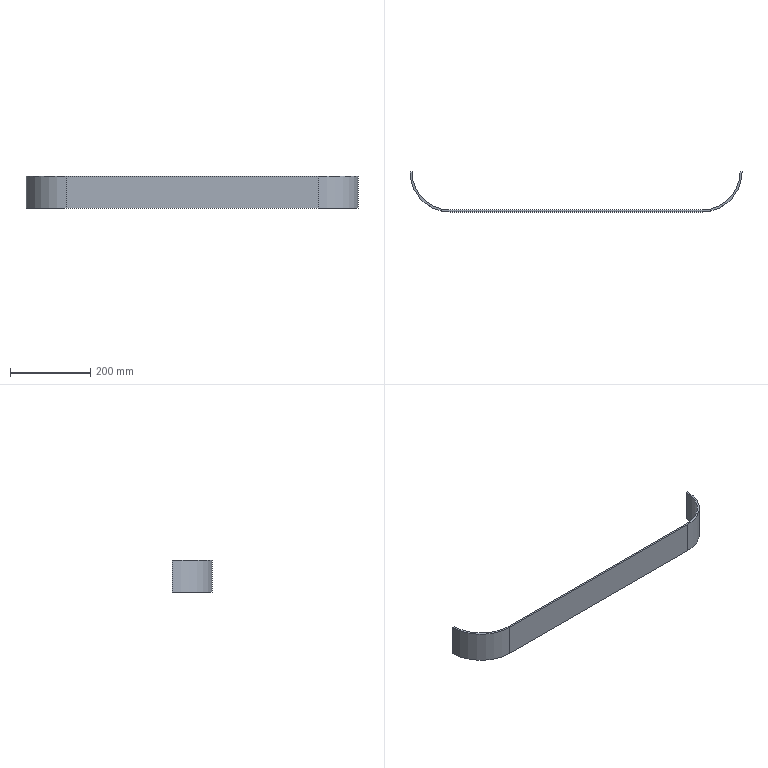Part | NX | features BREP 1 | 1 solid | 10 faces | box 830 x 100 x 80 mm | volume 374522 mm3 | plane 6 | cylinder 4 | commonest cylinder face diameters 190 x2 200 x2
STEP:
#1=CARTESIAN_POINT('',(-315.,-5.,80.));
#2=VERTEX_POINT('',#1);
#3=CARTESIAN_POINT('',(-415.,95.,80.));
#4=VERTEX_POINT('',#3);
#5=CARTESIAN_POINT('',(-315.,95.,80.));
#6=DIRECTION('',(0.,0.,-1.));
#7=DIRECTION('',(1.,0.,0.));
#8=AXIS2_PLACEMENT_3D('',#5,#6,#7);
#9=CIRCLE('',#8,100.);
#10=EDGE_CURVE('',#2,#4,#9,.T.);
#11=ORIENTED_EDGE('',*,*,#10,.F.);
#12=CARTESIAN_POINT('',(315.,-5.,80.));
#13=VERTEX_POINT('',#12);
#14=CARTESIAN_POINT('',(-315.,-5.,80.));
#15=DIRECTION('',(-1.,0.,0.));
#16=VECTOR('',#15,1000.);
#17=LINE('',#14,#16);
#18=EDGE_CURVE('',#13,#2,#17,.T.);
#19=ORIENTED_EDGE('',*,*,#18,.F.);
#20=CARTESIAN_POINT('',(415.,95.,80.));
#21=VERTEX_POINT('',#20);
#22=CARTESIAN_POINT('',(315.,95.,80.));
#23=DIRECTION('',(0.,0.,-1.));
#24=DIRECTION('',(1.,0.,0.));
#25=AXIS2_PLACEMENT_3D('',#22,#23,#24);
#26=CIRCLE('',#25,100.);
#27=EDGE_CURVE('',#21,#13,#26,.T.);
#28=ORIENTED_EDGE('',*,*,#27,.F.);
#29=CARTESIAN_POINT('',(410.,95.,80.));
#30=VERTEX_POINT('',#29);
#31=CARTESIAN_POINT('',(410.,95.,80.));
#32=DIRECTION('',(1.,0.,0.));
#33=VECTOR('',#32,1000.);
#34=LINE('',#31,#33);
#35=EDGE_CURVE('',#30,#21,#34,.T.);
#36=ORIENTED_EDGE('',*,*,#35,.F.);
#37=CARTESIAN_POINT('',(315.,0.,80.));
#38=VERTEX_POINT('',#37);
#39=CARTESIAN_POINT('',(315.,95.,80.));
#40=DIRECTION('',(0.,0.,-1.));
#41=DIRECTION('',(-1.,0.,0.));
#42=AXIS2_PLACEMENT_3D('',#39,#40,#41);
#43=CIRCLE('',#42,95.);
#44=EDGE_CURVE('',#30,#38,#43,.T.);
#45=ORIENTED_EDGE('',*,*,#44,.T.);
#46=CARTESIAN_POINT('',(-315.,0.,80.));
#47=VERTEX_POINT('',#46);
#48=CARTESIAN_POINT('',(-315.,0.,80.));
#49=DIRECTION('',(-1.,0.,0.));
#50=VECTOR('',#49,1000.);
#51=LINE('',#48,#50);
#52=EDGE_CURVE('',#38,#47,#51,.T.);
#53=ORIENTED_EDGE('',*,*,#52,.T.);
#54=CARTESIAN_POINT('',(-410.,95.,80.));
#55=VERTEX_POINT('',#54);
#56=CARTESIAN_POINT('',(-315.,95.,80.));
#57=DIRECTION('',(0.,0.,-1.));
#58=DIRECTION('',(1.,0.,0.));
#59=AXIS2_PLACEMENT_3D('',#56,#57,#58);
#60=CIRCLE('',#59,95.);
#61=EDGE_CURVE('',#47,#55,#60,.T.);
#62=ORIENTED_EDGE('',*,*,#61,.T.);
#63=CARTESIAN_POINT('',(-415.,95.,80.));
#64=DIRECTION('',(1.,0.,0.));
#65=VECTOR('',#64,1000.);
#66=LINE('',#63,#65);
#67=EDGE_CURVE('',#4,#55,#66,.T.);
#68=ORIENTED_EDGE('',*,*,#67,.F.);
#69=EDGE_LOOP('',(#11,#19,#28,#36,#45,#53,#62,#68));
#70=FACE_BOUND('',#69,.T.);
#71=CARTESIAN_POINT('',(-315.,0.,80.));
#72=DIRECTION('',(0.,0.,1.));
#73=DIRECTION('',(1.,0.,0.));
#74=AXIS2_PLACEMENT_3D('',#71,#72,#73);
#75=PLANE('',#74);
#76=ADVANCED_FACE('',(#70),#75,.T.);
#77=CARTESIAN_POINT('',(-315.,0.,0.));
#78=VERTEX_POINT('',#77);
#79=CARTESIAN_POINT('',(-410.,95.,0.));
#80=VERTEX_POINT('',#79);
#81=CARTESIAN_POINT('',(-315.,95.,0.));
#82=DIRECTION('',(0.,0.,-1.));
#83=DIRECTION('',(1.,0.,0.));
#84=AXIS2_PLACEMENT_3D('',#81,#82,#83);
#85=CIRCLE('',#84,95.);
#86=EDGE_CURVE('',#78,#80,#85,.T.);
#87=ORIENTED_EDGE('',*,*,#86,.F.);
#88=CARTESIAN_POINT('',(315.,0.,0.));
#89=VERTEX_POINT('',#88);
#90=CARTESIAN_POINT('',(-315.,0.,0.));
#91=DIRECTION('',(-1.,0.,0.));
#92=VECTOR('',#91,1000.);
#93=LINE('',#90,#92);
#94=EDGE_CURVE('',#89,#78,#93,.T.);
#95=ORIENTED_EDGE('',*,*,#94,.F.);
#96=CARTESIAN_POINT('',(410.,95.,0.));
#97=VERTEX_POINT('',#96);
#98=CARTESIAN_POINT('',(315.,95.,0.));
#99=DIRECTION('',(0.,0.,-1.));
#100=DIRECTION('',(-1.,0.,0.));
#101=AXIS2_PLACEMENT_3D('',#98,#99,#100);
#102=CIRCLE('',#101,95.);
#103=EDGE_CURVE('',#97,#89,#102,.T.);
#104=ORIENTED_EDGE('',*,*,#103,.F.);
#105=CARTESIAN_POINT('',(415.,95.,0.));
#106=VERTEX_POINT('',#105);
#107=CARTESIAN_POINT('',(410.,95.,0.));
#108=DIRECTION('',(1.,0.,0.));
#109=VECTOR('',#108,1000.);
#110=LINE('',#107,#109);
#111=EDGE_CURVE('',#97,#106,#110,.T.);
#112=ORIENTED_EDGE('',*,*,#111,.T.);
#113=CARTESIAN_POINT('',(315.,-5.,0.));
#114=VERTEX_POINT('',#113);
#115=CARTESIAN_POINT('',(315.,95.,0.));
#116=DIRECTION('',(0.,0.,-1.));
#117=DIRECTION('',(1.,0.,0.));
#118=AXIS2_PLACEMENT_3D('',#115,#116,#117);
#119=CIRCLE('',#118,100.);
#120=EDGE_CURVE('',#106,#114,#119,.T.);
#121=ORIENTED_EDGE('',*,*,#120,.T.);
#122=CARTESIAN_POINT('',(-315.,-5.,0.));
#123=VERTEX_POINT('',#122);
#124=CARTESIAN_POINT('',(-315.,-5.,0.));
#125=DIRECTION('',(-1.,0.,0.));
#126=VECTOR('',#125,1000.);
#127=LINE('',#124,#126);
#128=EDGE_CURVE('',#114,#123,#127,.T.);
#129=ORIENTED_EDGE('',*,*,#128,.T.);
#130=CARTESIAN_POINT('',(-415.,95.,0.));
#131=VERTEX_POINT('',#130);
#132=CARTESIAN_POINT('',(-315.,95.,0.));
#133=DIRECTION('',(0.,0.,-1.));
#134=DIRECTION('',(1.,0.,0.));
#135=AXIS2_PLACEMENT_3D('',#132,#133,#134);
#136=CIRCLE('',#135,100.);
#137=EDGE_CURVE('',#123,#131,#136,.T.);
#138=ORIENTED_EDGE('',*,*,#137,.T.);
#139=CARTESIAN_POINT('',(-415.,95.,0.));
#140=DIRECTION('',(1.,0.,0.));
#141=VECTOR('',#140,1000.);
#142=LINE('',#139,#141);
#143=EDGE_CURVE('',#131,#80,#142,.T.);
#144=ORIENTED_EDGE('',*,*,#143,.T.);
#145=EDGE_LOOP('',(#87,#95,#104,#112,#121,#129,#138,#144));
#146=FACE_BOUND('',#145,.T.);
#147=CARTESIAN_POINT('',(-315.,-5.,0.));
#148=DIRECTION('',(0.,0.,-1.));
#149=DIRECTION('',(-1.,0.,0.));
#150=AXIS2_PLACEMENT_3D('',#147,#148,#149);
#151=PLANE('',#150);
#152=ADVANCED_FACE('',(#146),#151,.T.);
#153=ORIENTED_EDGE('',*,*,#86,.T.);
#154=CARTESIAN_POINT('',(-410.,95.,80.));
#155=DIRECTION('',(0.,0.,-1.));
#156=VECTOR('',#155,1000.);
#157=LINE('',#154,#156);
#158=EDGE_CURVE('',#55,#80,#157,.T.);
#159=ORIENTED_EDGE('',*,*,#158,.F.);
#160=ORIENTED_EDGE('',*,*,#61,.F.);
#161=CARTESIAN_POINT('',(-315.,0.,80.));
#162=DIRECTION('',(0.,0.,-1.));
#163=VECTOR('',#162,1000.);
#164=LINE('',#161,#163);
#165=EDGE_CURVE('',#47,#78,#164,.T.);
#166=ORIENTED_EDGE('',*,*,#165,.T.);
#167=EDGE_LOOP('',(#153,#159,#160,#166));
#168=FACE_BOUND('',#167,.T.);
#169=CARTESIAN_POINT('',(-315.,95.,80.));
#170=DIRECTION('',(0.,0.,-1.));
#171=DIRECTION('',(-1.,0.,0.));
#172=AXIS2_PLACEMENT_3D('',#169,#170,#171);
#173=CYLINDRICAL_SURFACE('',#172,95.);
#174=ADVANCED_FACE('',(#168),#173,.F.);
#175=ORIENTED_EDGE('',*,*,#143,.F.);
#176=CARTESIAN_POINT('',(-415.,95.,80.));
#177=DIRECTION('',(0.,0.,-1.));
#178=VECTOR('',#177,1000.);
#179=LINE('',#176,#178);
#180=EDGE_CURVE('',#4,#131,#179,.T.);
#181=ORIENTED_EDGE('',*,*,#180,.F.);
#182=ORIENTED_EDGE('',*,*,#67,.T.);
#183=ORIENTED_EDGE('',*,*,#158,.T.);
#184=EDGE_LOOP('',(#175,#181,#182,#183));
#185=FACE_BOUND('',#184,.T.);
#186=CARTESIAN_POINT('',(-415.,95.,80.));
#187=DIRECTION('',(0.,1.,0.));
#188=DIRECTION('',(0.,0.,1.));
#189=AXIS2_PLACEMENT_3D('',#186,#187,#188);
#190=PLANE('',#189);
#191=ADVANCED_FACE('',(#185),#190,.T.);
#192=ORIENTED_EDGE('',*,*,#137,.F.);
#193=CARTESIAN_POINT('',(-315.,-5.,80.));
#194=DIRECTION('',(0.,0.,-1.));
#195=VECTOR('',#194,1000.);
#196=LINE('',#193,#195);
#197=EDGE_CURVE('',#2,#123,#196,.T.);
#198=ORIENTED_EDGE('',*,*,#197,.F.);
#199=ORIENTED_EDGE('',*,*,#10,.T.);
#200=ORIENTED_EDGE('',*,*,#180,.T.);
#201=EDGE_LOOP('',(#192,#198,#199,#200));
#202=FACE_BOUND('',#201,.T.);
#203=CARTESIAN_POINT('',(-315.,95.,80.));
#204=DIRECTION('',(0.,0.,-1.));
#205=DIRECTION('',(-1.,0.,0.));
#206=AXIS2_PLACEMENT_3D('',#203,#204,#205);
#207=CYLINDRICAL_SURFACE('',#206,100.);
#208=ADVANCED_FACE('',(#202),#207,.T.);
#209=ORIENTED_EDGE('',*,*,#128,.F.);
#210=CARTESIAN_POINT('',(315.,-5.,80.));
#211=DIRECTION('',(0.,0.,-1.));
#212=VECTOR('',#211,1000.);
#213=LINE('',#210,#212);
#214=EDGE_CURVE('',#13,#114,#213,.T.);
#215=ORIENTED_EDGE('',*,*,#214,.F.);
#216=ORIENTED_EDGE('',*,*,#18,.T.);
#217=ORIENTED_EDGE('',*,*,#197,.T.);
#218=EDGE_LOOP('',(#209,#215,#216,#217));
#219=FACE_BOUND('',#218,.T.);
#220=CARTESIAN_POINT('',(-315.,-5.,80.));
#221=DIRECTION('',(0.,-1.,0.));
#222=DIRECTION('',(0.,0.,-1.));
#223=AXIS2_PLACEMENT_3D('',#220,#221,#222);
#224=PLANE('',#223);
#225=ADVANCED_FACE('',(#219),#224,.T.);
#226=ORIENTED_EDGE('',*,*,#120,.F.);
#227=CARTESIAN_POINT('',(415.,95.,80.));
#228=DIRECTION('',(0.,0.,-1.));
#229=VECTOR('',#228,1000.);
#230=LINE('',#227,#229);
#231=EDGE_CURVE('',#21,#106,#230,.T.);
#232=ORIENTED_EDGE('',*,*,#231,.F.);
#233=ORIENTED_EDGE('',*,*,#27,.T.);
#234=ORIENTED_EDGE('',*,*,#214,.T.);
#235=EDGE_LOOP('',(#226,#232,#233,#234));
#236=FACE_BOUND('',#235,.T.);
#237=CARTESIAN_POINT('',(315.,95.,80.));
#238=DIRECTION('',(0.,0.,-1.));
#239=DIRECTION('',(-1.,0.,0.));
#240=AXIS2_PLACEMENT_3D('',#237,#238,#239);
#241=CYLINDRICAL_SURFACE('',#240,100.);
#242=ADVANCED_FACE('',(#236),#241,.T.);
#243=ORIENTED_EDGE('',*,*,#111,.F.);
#244=CARTESIAN_POINT('',(410.,95.,80.));
#245=DIRECTION('',(0.,0.,-1.));
#246=VECTOR('',#245,1000.);
#247=LINE('',#244,#246);
#248=EDGE_CURVE('',#30,#97,#247,.T.);
#249=ORIENTED_EDGE('',*,*,#248,.F.);
#250=ORIENTED_EDGE('',*,*,#35,.T.);
#251=ORIENTED_EDGE('',*,*,#231,.T.);
#252=EDGE_LOOP('',(#243,#249,#250,#251));
#253=FACE_BOUND('',#252,.T.);
#254=CARTESIAN_POINT('',(410.,95.,80.));
#255=DIRECTION('',(0.,1.,0.));
#256=DIRECTION('',(0.,0.,1.));
#257=AXIS2_PLACEMENT_3D('',#254,#255,#256);
#258=PLANE('',#257);
#259=ADVANCED_FACE('',(#253),#258,.T.);
#260=ORIENTED_EDGE('',*,*,#103,.T.);
#261=CARTESIAN_POINT('',(315.,0.,80.));
#262=DIRECTION('',(0.,0.,-1.));
#263=VECTOR('',#262,1000.);
#264=LINE('',#261,#263);
#265=EDGE_CURVE('',#38,#89,#264,.T.);
#266=ORIENTED_EDGE('',*,*,#265,.F.);
#267=ORIENTED_EDGE('',*,*,#44,.F.);
#268=ORIENTED_EDGE('',*,*,#248,.T.);
#269=EDGE_LOOP('',(#260,#266,#267,#268));
#270=FACE_BOUND('',#269,.T.);
#271=CARTESIAN_POINT('',(315.,95.,80.));
#272=DIRECTION('',(0.,0.,-1.));
#273=DIRECTION('',(-1.,0.,0.));
#274=AXIS2_PLACEMENT_3D('',#271,#272,#273);
#275=CYLINDRICAL_SURFACE('',#274,95.);
#276=ADVANCED_FACE('',(#270),#275,.F.);
#277=ORIENTED_EDGE('',*,*,#94,.T.);
#278=ORIENTED_EDGE('',*,*,#165,.F.);
#279=ORIENTED_EDGE('',*,*,#52,.F.);
#280=ORIENTED_EDGE('',*,*,#265,.T.);
#281=EDGE_LOOP('',(#277,#278,#279,#280));
#282=FACE_BOUND('',#281,.T.);
#283=CARTESIAN_POINT('',(-315.,0.,80.));
#284=DIRECTION('',(0.,-1.,0.));
#285=DIRECTION('',(0.,0.,-1.));
#286=AXIS2_PLACEMENT_3D('',#283,#284,#285);
#287=PLANE('',#286);
#288=ADVANCED_FACE('',(#282),#287,.F.);
#289=CLOSED_SHELL('',(#76,#152,#174,#191,#208,#225,#242,#259,#276,#288));
#290=MANIFOLD_SOLID_BREP('',#289);
#291=(LENGTH_UNIT()NAMED_UNIT(*)SI_UNIT(.MILLI.,.METRE.));
#292=UNCERTAINTY_MEASURE_WITH_UNIT(LENGTH_MEASURE(0.00001),#291,'','');
#293=(NAMED_UNIT(*)PLANE_ANGLE_UNIT()SI_UNIT($,.RADIAN.));
#294=(NAMED_UNIT(*)SI_UNIT($,.STERADIAN.)SOLID_ANGLE_UNIT());
#295=(GEOMETRIC_REPRESENTATION_CONTEXT(3)GLOBAL_UNCERTAINTY_ASSIGNED_CONTEXT((#292))GLOBAL_UNIT_ASSIGNED_CONTEXT((#291,#293,#294))REPRESENTATION_CONTEXT('',''));
#296=ADVANCED_BREP_SHAPE_REPRESENTATION('',(#290),#295);